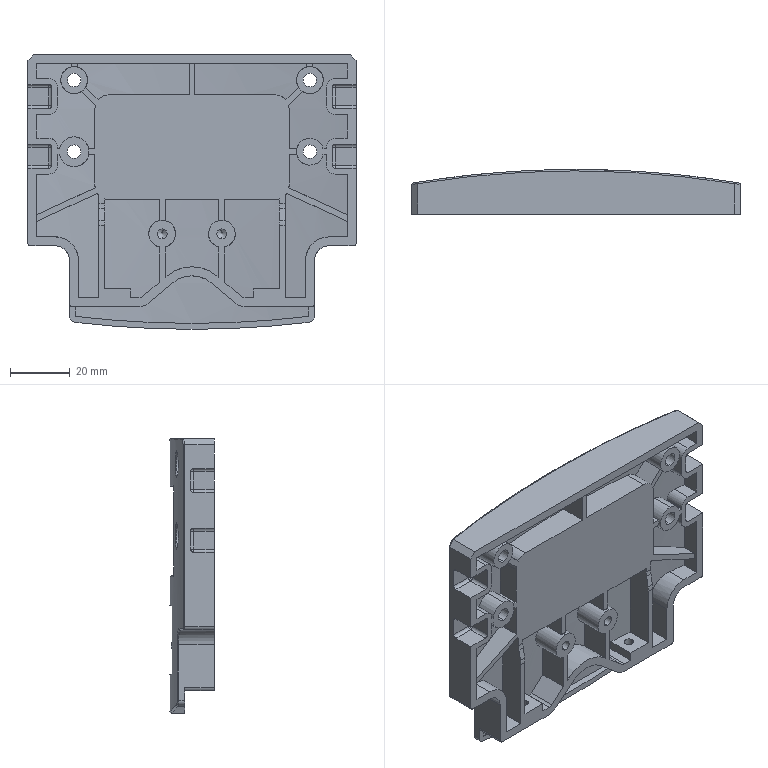Part | SolidWorks | features BaseBody 1 | 1 solid | 342 faces | box 110 x 15 x 92 mm | volume 55640 mm3 | plane 144 | cylinder 128 | spline 66 | cone 4 | commonest cylinder face diameters 2 x24 9 x21 650 x11 1 x10 3.3 x8 4 x8